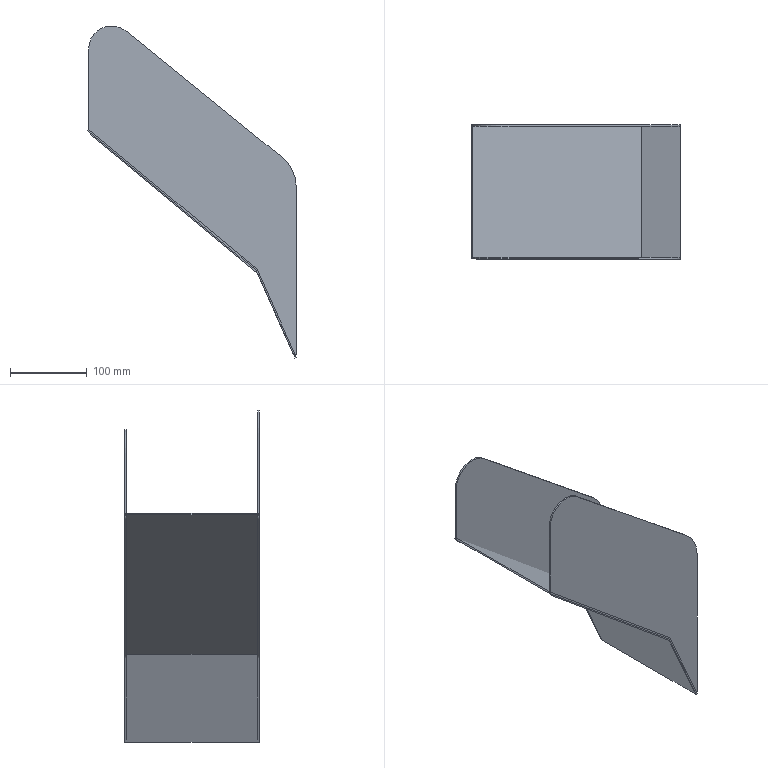Part | STEP file | COMPOUND | 3 solids | 32 faces | box 271.977 x 175 x 432.84 mm | volume 323014 mm3 | plane 22 | cylinder 10 | commonest cylinder face diameters 20 x4 4 x2 60 x2 100 x2